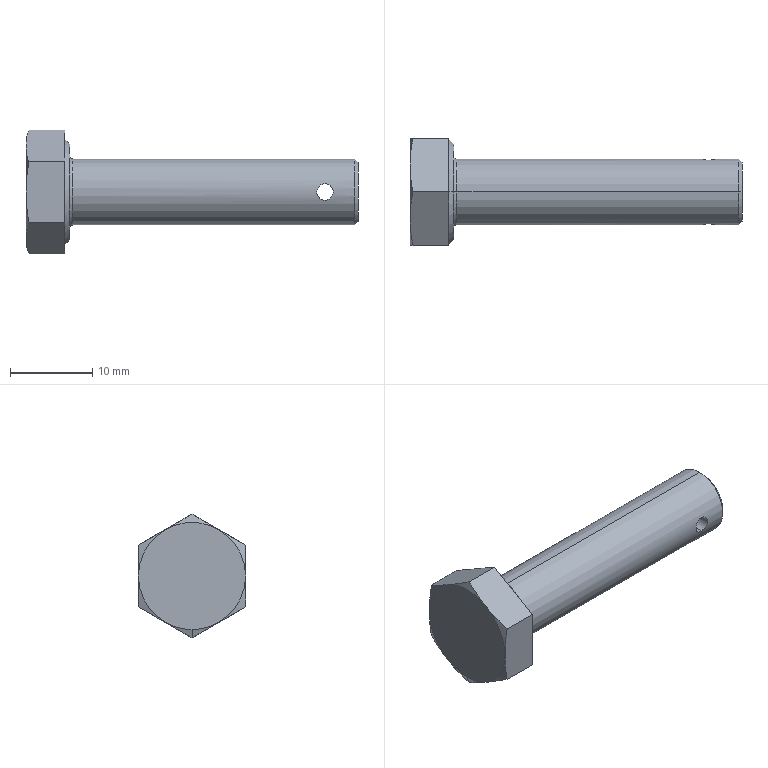Part | STEP file | hex bolts split pin hole-fine pitch-ab gb_PreviewCfg | 1 solid | 27 faces | box 40.3 x 13 x 15.011 mm | volume 2490 mm3 | cone 11 | plane 10 | cylinder 4 | torus 2 | commonest cylinder face diameters 2 x2 8 x2
STEP:
#1=CARTESIAN_POINT('',(5.7,0.,4.));
#2=VERTEX_POINT('',#1);
#3=CARTESIAN_POINT('',(5.7,0.,-4.));
#4=VERTEX_POINT('',#3);
#5=CARTESIAN_POINT('',(5.7,0.,0.));
#6=DIRECTION('',(1.,0.,0.));
#7=DIRECTION('',(0.,0.,-1.));
#8=AXIS2_PLACEMENT_3D('',#5,#6,#7);
#9=CIRCLE('',#8,4.);
#10=EDGE_CURVE('',#2,#4,#9,.T.);
#11=ORIENTED_EDGE('',*,*,#10,.F.);
#12=CARTESIAN_POINT('',(5.3,0.,4.4));
#13=VERTEX_POINT('',#12);
#14=CARTESIAN_POINT('',(5.7,0.,4.4));
#15=DIRECTION('',(0.,1.,0.));
#16=DIRECTION('',(0.,0.,1.));
#17=AXIS2_PLACEMENT_3D('',#14,#15,#16);
#18=CIRCLE('',#17,0.4);
#19=EDGE_CURVE('',#2,#13,#18,.T.);
#20=ORIENTED_EDGE('',*,*,#19,.T.);
#21=CARTESIAN_POINT('',(5.3,0.,-4.4));
#22=VERTEX_POINT('',#21);
#23=CARTESIAN_POINT('',(5.3,0.,0.));
#24=DIRECTION('',(-1.,0.,0.));
#25=DIRECTION('',(0.,0.,-1.));
#26=AXIS2_PLACEMENT_3D('',#23,#24,#25);
#27=CIRCLE('',#26,4.4);
#28=EDGE_CURVE('',#22,#13,#27,.T.);
#29=ORIENTED_EDGE('',*,*,#28,.F.);
#30=CARTESIAN_POINT('',(5.7,0.,-4.4));
#31=DIRECTION('',(0.,-1.,0.));
#32=DIRECTION('',(0.,0.,-1.));
#33=AXIS2_PLACEMENT_3D('',#30,#31,#32);
#34=CIRCLE('',#33,0.4);
#35=EDGE_CURVE('',#4,#22,#34,.T.);
#36=ORIENTED_EDGE('',*,*,#35,.F.);
#37=EDGE_LOOP('',(#11,#20,#29,#36));
#38=FACE_OUTER_BOUND('',#37,.T.);
#39=CARTESIAN_POINT('',(5.7,0.,0.));
#40=DIRECTION('',(1.,0.,0.));
#41=DIRECTION('',(0.,0.,-1.));
#42=AXIS2_PLACEMENT_3D('',#39,#40,#41);
#43=TOROIDAL_SURFACE('',#42,4.4,0.4);
#44=ADVANCED_FACE('',(#38),#43,.F.);
#45=CARTESIAN_POINT('',(36.3,-3.873,-1.));
#46=VERTEX_POINT('',#45);
#47=CARTESIAN_POINT('',(36.3,-3.873,1.));
#48=VERTEX_POINT('',#47);
#49=CARTESIAN_POINT('',(36.3,-3.873,-1.));
#50=CARTESIAN_POINT('',(36.169,-3.873,-1.));
#51=CARTESIAN_POINT('',(36.037,-3.88,-0.9736));
#52=CARTESIAN_POINT('',(35.796,-3.904,-0.8737));
#53=CARTESIAN_POINT('',(35.685,-3.92,-0.7996));
#54=CARTESIAN_POINT('',(35.501,-3.954,-0.6153));
#55=CARTESIAN_POINT('',(35.427,-3.97,-0.5057));
#56=CARTESIAN_POINT('',(35.326,-3.993,-0.2624));
#57=CARTESIAN_POINT('',(35.3,-4.,-0.1322));
#58=CARTESIAN_POINT('',(35.3,-4.,0.1316));
#59=CARTESIAN_POINT('',(35.326,-3.993,0.2627));
#60=CARTESIAN_POINT('',(35.426,-3.97,0.5039));
#61=CARTESIAN_POINT('',(35.501,-3.954,0.615));
#62=CARTESIAN_POINT('',(35.684,-3.921,0.7986));
#63=CARTESIAN_POINT('',(35.795,-3.904,0.873));
#64=CARTESIAN_POINT('',(36.036,-3.88,0.9733));
#65=CARTESIAN_POINT('',(36.167,-3.873,1.));
#66=CARTESIAN_POINT('',(36.3,-3.873,1.));
#67=B_SPLINE_CURVE_WITH_KNOTS('',3,(#49,#50,#51,#52,#53,#54,#55,#56,#57,#58,#59,#60,#61,#62,#63,#64,#65,#66),.UNSPECIFIED.,.F.,.F.,(4,2,2,2,2,2,2,2,4),(0.003139,0.003531,0.003923,0.004316,0.004708,0.0051,0.005492,0.005885,0.006277),.UNSPECIFIED.);
#68=EDGE_CURVE('',#46,#48,#67,.T.);
#69=ORIENTED_EDGE('',*,*,#68,.F.);
#70=CARTESIAN_POINT('',(36.3,3.873,-1.));
#71=VERTEX_POINT('',#70);
#72=CARTESIAN_POINT('',(36.3,-6.5,-1.));
#73=DIRECTION('',(0.,1.,0.));
#74=VECTOR('',#73,1000.);
#75=LINE('',#72,#74);
#76=EDGE_CURVE('',#46,#71,#75,.T.);
#77=ORIENTED_EDGE('',*,*,#76,.T.);
#78=CARTESIAN_POINT('',(36.3,3.873,1.));
#79=VERTEX_POINT('',#78);
#80=CARTESIAN_POINT('',(36.3,3.873,1.));
#81=CARTESIAN_POINT('',(36.167,3.873,1.));
#82=CARTESIAN_POINT('',(36.037,3.88,0.9737));
#83=CARTESIAN_POINT('',(35.795,3.904,0.8731));
#84=CARTESIAN_POINT('',(35.685,3.921,0.7988));
#85=CARTESIAN_POINT('',(35.501,3.954,0.6151));
#86=CARTESIAN_POINT('',(35.426,3.97,0.5039));
#87=CARTESIAN_POINT('',(35.327,3.993,0.2634));
#88=CARTESIAN_POINT('',(35.3,4.,0.1315));
#89=CARTESIAN_POINT('',(35.3,4.,-0.1306));
#90=CARTESIAN_POINT('',(35.326,3.993,-0.2619));
#91=CARTESIAN_POINT('',(35.427,3.97,-0.5048));
#92=CARTESIAN_POINT('',(35.5,3.954,-0.6147));
#93=CARTESIAN_POINT('',(35.686,3.92,-0.7999));
#94=CARTESIAN_POINT('',(35.796,3.904,-0.8735));
#95=CARTESIAN_POINT('',(36.037,3.88,-0.9737));
#96=CARTESIAN_POINT('',(36.169,3.873,-1.));
#97=CARTESIAN_POINT('',(36.3,3.873,-1.));
#98=B_SPLINE_CURVE_WITH_KNOTS('',3,(#80,#81,#82,#83,#84,#85,#86,#87,#88,#89,#90,#91,#92,#93,#94,#95,#96,#97),.UNSPECIFIED.,.F.,.F.,(4,2,2,2,2,2,2,2,4),(0.,0.0003924,0.0007847,0.001177,0.001569,0.001962,0.002354,0.002747,0.003139),.UNSPECIFIED.);
#99=EDGE_CURVE('',#79,#71,#98,.T.);
#100=ORIENTED_EDGE('',*,*,#99,.F.);
#101=CARTESIAN_POINT('',(36.3,-6.5,1.));
#102=DIRECTION('',(0.,1.,0.));
#103=VECTOR('',#102,1000.);
#104=LINE('',#101,#103);
#105=EDGE_CURVE('',#48,#79,#104,.T.);
#106=ORIENTED_EDGE('',*,*,#105,.F.);
#107=EDGE_LOOP('',(#69,#77,#100,#106));
#108=FACE_OUTER_BOUND('',#107,.T.);
#109=CARTESIAN_POINT('',(36.3,-6.5,0.));
#110=DIRECTION('',(0.,1.,0.));
#111=DIRECTION('',(0.,0.,1.));
#112=AXIS2_PLACEMENT_3D('',#109,#110,#111);
#113=CYLINDRICAL_SURFACE('',#112,1.);
#114=ADVANCED_FACE('',(#108),#113,.F.);
#115=CARTESIAN_POINT('',(40.3,0.,-3.6));
#116=VERTEX_POINT('',#115);
#117=CARTESIAN_POINT('',(40.3,0.,3.6));
#118=VERTEX_POINT('',#117);
#119=CARTESIAN_POINT('',(40.3,0.,0.));
#120=DIRECTION('',(1.,0.,0.));
#121=DIRECTION('',(0.,0.,-1.));
#122=AXIS2_PLACEMENT_3D('',#119,#120,#121);
#123=CIRCLE('',#122,3.6);
#124=EDGE_CURVE('',#116,#118,#123,.T.);
#125=ORIENTED_EDGE('',*,*,#124,.F.);
#126=CARTESIAN_POINT('',(39.9,0.,-4.));
#127=VERTEX_POINT('',#126);
#128=CARTESIAN_POINT('',(40.3,0.,-3.6));
#129=DIRECTION('',(-0.7071,0.,-0.7071));
#130=VECTOR('',#129,1000.);
#131=LINE('',#128,#130);
#132=EDGE_CURVE('',#116,#127,#131,.T.);
#133=ORIENTED_EDGE('',*,*,#132,.T.);
#134=CARTESIAN_POINT('',(39.9,0.,4.));
#135=VERTEX_POINT('',#134);
#136=CARTESIAN_POINT('',(39.9,0.,0.));
#137=DIRECTION('',(-1.,0.,0.));
#138=DIRECTION('',(0.,0.,-1.));
#139=AXIS2_PLACEMENT_3D('',#136,#137,#138);
#140=CIRCLE('',#139,4.);
#141=EDGE_CURVE('',#135,#127,#140,.T.);
#142=ORIENTED_EDGE('',*,*,#141,.F.);
#143=CARTESIAN_POINT('',(40.3,0.,3.6));
#144=DIRECTION('',(-0.7071,0.,0.7071));
#145=VECTOR('',#144,1000.);
#146=LINE('',#143,#145);
#147=EDGE_CURVE('',#118,#135,#146,.T.);
#148=ORIENTED_EDGE('',*,*,#147,.F.);
#149=EDGE_LOOP('',(#125,#133,#142,#148));
#150=FACE_OUTER_BOUND('',#149,.T.);
#151=CARTESIAN_POINT('',(40.3,0.,0.));
#152=DIRECTION('',(-1.,0.,0.));
#153=DIRECTION('',(0.,0.,1.));
#154=AXIS2_PLACEMENT_3D('',#151,#152,#153);
#155=CONICAL_SURFACE('',#154,3.6,0.7854);
#156=ADVANCED_FACE('',(#150),#155,.T.);
#157=ORIENTED_EDGE('',*,*,#99,.T.);
#158=CARTESIAN_POINT('',(36.3,3.873,-1.));
#159=CARTESIAN_POINT('',(36.431,3.873,-1.));
#160=CARTESIAN_POINT('',(36.563,3.88,-0.9736));
#161=CARTESIAN_POINT('',(36.804,3.904,-0.8737));
#162=CARTESIAN_POINT('',(36.915,3.92,-0.7996));
#163=CARTESIAN_POINT('',(37.099,3.954,-0.6153));
#164=CARTESIAN_POINT('',(37.173,3.97,-0.5057));
#165=CARTESIAN_POINT('',(37.274,3.993,-0.2624));
#166=CARTESIAN_POINT('',(37.3,4.,-0.1322));
#167=CARTESIAN_POINT('',(37.3,4.,0.1316));
#168=CARTESIAN_POINT('',(37.274,3.993,0.2627));
#169=CARTESIAN_POINT('',(37.174,3.97,0.5039));
#170=CARTESIAN_POINT('',(37.099,3.954,0.615));
#171=CARTESIAN_POINT('',(36.916,3.921,0.7986));
#172=CARTESIAN_POINT('',(36.805,3.904,0.873));
#173=CARTESIAN_POINT('',(36.564,3.88,0.9733));
#174=CARTESIAN_POINT('',(36.433,3.873,1.));
#175=CARTESIAN_POINT('',(36.3,3.873,1.));
#176=B_SPLINE_CURVE_WITH_KNOTS('',3,(#158,#159,#160,#161,#162,#163,#164,#165,#166,#167,#168,#169,#170,#171,#172,#173,#174,#175),.UNSPECIFIED.,.F.,.F.,(4,2,2,2,2,2,2,2,4),(0.003139,0.003531,0.003923,0.004316,0.004708,0.0051,0.005492,0.005885,0.006277),.UNSPECIFIED.);
#177=EDGE_CURVE('',#71,#79,#176,.T.);
#178=ORIENTED_EDGE('',*,*,#177,.T.);
#179=EDGE_LOOP('',(#157,#178));
#180=FACE_BOUND('',#179,.T.);
#181=ORIENTED_EDGE('',*,*,#141,.T.);
#182=CARTESIAN_POINT('',(40.3,0.,-4.));
#183=DIRECTION('',(-1.,0.,0.));
#184=VECTOR('',#183,1000.);
#185=LINE('',#182,#184);
#186=EDGE_CURVE('',#127,#4,#185,.T.);
#187=ORIENTED_EDGE('',*,*,#186,.T.);
#188=CARTESIAN_POINT('',(5.7,0.,0.));
#189=DIRECTION('',(1.,0.,0.));
#190=DIRECTION('',(0.,0.,-1.));
#191=AXIS2_PLACEMENT_3D('',#188,#189,#190);
#192=CIRCLE('',#191,4.);
#193=EDGE_CURVE('',#4,#2,#192,.T.);
#194=ORIENTED_EDGE('',*,*,#193,.T.);
#195=CARTESIAN_POINT('',(40.3,0.,4.));
#196=DIRECTION('',(-1.,0.,0.));
#197=VECTOR('',#196,1000.);
#198=LINE('',#195,#197);
#199=EDGE_CURVE('',#135,#2,#198,.T.);
#200=ORIENTED_EDGE('',*,*,#199,.F.);
#201=EDGE_LOOP('',(#181,#187,#194,#200));
#202=FACE_OUTER_BOUND('',#201,.T.);
#203=CARTESIAN_POINT('',(40.3,0.,0.));
#204=DIRECTION('',(-1.,0.,0.));
#205=DIRECTION('',(0.,0.,1.));
#206=AXIS2_PLACEMENT_3D('',#203,#204,#205);
#207=CYLINDRICAL_SURFACE('',#206,4.);
#208=ADVANCED_FACE('',(#180,#202),#207,.T.);
#209=CARTESIAN_POINT('',(0.,-3.25,-5.629));
#210=VERTEX_POINT('',#209);
#211=CARTESIAN_POINT('',(0.,0.,-6.5));
#212=VERTEX_POINT('',#211);
#213=CARTESIAN_POINT('',(0.,0.,0.));
#214=DIRECTION('',(1.,0.,0.));
#215=DIRECTION('',(0.,0.,-1.));
#216=AXIS2_PLACEMENT_3D('',#213,#214,#215);
#217=CIRCLE('',#216,6.5);
#218=EDGE_CURVE('',#210,#212,#217,.T.);
#219=ORIENTED_EDGE('',*,*,#218,.T.);
#220=CARTESIAN_POINT('',(0.366,0.,-7.506));
#221=VERTEX_POINT('',#220);
#222=CARTESIAN_POINT('',(0.,0.,-6.5));
#223=DIRECTION('',(0.342,0.,-0.9397));
#224=VECTOR('',#223,1000.);
#225=LINE('',#222,#224);
#226=EDGE_CURVE('',#212,#221,#225,.T.);
#227=ORIENTED_EDGE('',*,*,#226,.T.);
#228=CARTESIAN_POINT('',(0.366,0.,-7.506));
#229=CARTESIAN_POINT('',(0.2522,-0.5417,-7.193));
#230=CARTESIAN_POINT('',(0.1597,-1.083,-6.88));
#231=CARTESIAN_POINT('',(0.03346,-2.167,-6.255));
#232=CARTESIAN_POINT('',(0.,-2.708,-5.942));
#233=CARTESIAN_POINT('',(0.,-3.25,-5.629));
#234=B_SPLINE_CURVE_WITH_KNOTS('',3,(#228,#229,#230,#231,#232,#233),.UNSPECIFIED.,.F.,.F.,(4,2,4),(0.000000231,0.001877,0.003753),.UNSPECIFIED.);
#235=EDGE_CURVE('',#221,#210,#234,.T.);
#236=ORIENTED_EDGE('',*,*,#235,.T.);
#237=EDGE_LOOP('',(#219,#227,#236));
#238=FACE_OUTER_BOUND('',#237,.T.);
#239=CARTESIAN_POINT('',(0.,0.,0.));
#240=DIRECTION('',(1.,0.,0.));
#241=DIRECTION('',(0.,0.,-1.));
#242=AXIS2_PLACEMENT_3D('',#239,#240,#241);
#243=CONICAL_SURFACE('',#242,6.5,1.222);
#244=ADVANCED_FACE('',(#238),#243,.T.);
#245=CARTESIAN_POINT('',(5.3,0.,5.815));
#246=VERTEX_POINT('',#245);
#247=CARTESIAN_POINT('',(5.3,0.,-5.815));
#248=VERTEX_POINT('',#247);
#249=CARTESIAN_POINT('',(5.3,0.,0.));
#250=DIRECTION('',(-1.,0.,0.));
#251=DIRECTION('',(0.,0.,1.));
#252=AXIS2_PLACEMENT_3D('',#249,#250,#251);
#253=CIRCLE('',#252,5.815);
#254=EDGE_CURVE('',#246,#248,#253,.T.);
#255=ORIENTED_EDGE('',*,*,#254,.T.);
#256=CARTESIAN_POINT('',(4.7,0.,-6.415));
#257=VERTEX_POINT('',#256);
#258=CARTESIAN_POINT('',(4.7,0.,-6.415));
#259=DIRECTION('',(-0.7071,0.,-0.7071));
#260=VECTOR('',#259,1000.);
#261=LINE('',#258,#260);
#262=EDGE_CURVE('',#248,#257,#261,.T.);
#263=ORIENTED_EDGE('',*,*,#262,.T.);
#264=CARTESIAN_POINT('',(4.7,0.,6.415));
#265=VERTEX_POINT('',#264);
#266=CARTESIAN_POINT('',(4.7,0.,0.));
#267=DIRECTION('',(-1.,0.,0.));
#268=DIRECTION('',(0.,0.,1.));
#269=AXIS2_PLACEMENT_3D('',#266,#267,#268);
#270=CIRCLE('',#269,6.415);
#271=EDGE_CURVE('',#265,#257,#270,.T.);
#272=ORIENTED_EDGE('',*,*,#271,.F.);
#273=CARTESIAN_POINT('',(4.7,0.,6.415));
#274=DIRECTION('',(-0.7071,0.,0.7071));
#275=VECTOR('',#274,1000.);
#276=LINE('',#273,#275);
#277=EDGE_CURVE('',#246,#265,#276,.T.);
#278=ORIENTED_EDGE('',*,*,#277,.F.);
#279=EDGE_LOOP('',(#255,#263,#272,#278));
#280=FACE_OUTER_BOUND('',#279,.T.);
#281=CARTESIAN_POINT('',(4.7,0.,0.));
#282=DIRECTION('',(-1.,0.,0.));
#283=DIRECTION('',(0.,0.,1.));
#284=AXIS2_PLACEMENT_3D('',#281,#282,#283);
#285=CONICAL_SURFACE('',#284,6.415,0.7854);
#286=ADVANCED_FACE('',(#280),#285,.T.);
#287=ORIENTED_EDGE('',*,*,#28,.T.);
#288=CARTESIAN_POINT('',(5.3,0.,0.));
#289=DIRECTION('',(-1.,0.,0.));
#290=DIRECTION('',(0.,0.,-1.));
#291=AXIS2_PLACEMENT_3D('',#288,#289,#290);
#292=CIRCLE('',#291,4.4);
#293=EDGE_CURVE('',#13,#22,#292,.T.);
#294=ORIENTED_EDGE('',*,*,#293,.T.);
#295=EDGE_LOOP('',(#287,#294));
#296=FACE_BOUND('',#295,.T.);
#297=ORIENTED_EDGE('',*,*,#254,.F.);
#298=CARTESIAN_POINT('',(5.3,0.,0.));
#299=DIRECTION('',(-1.,0.,0.));
#300=DIRECTION('',(0.,0.,1.));
#301=AXIS2_PLACEMENT_3D('',#298,#299,#300);
#302=CIRCLE('',#301,5.815);
#303=EDGE_CURVE('',#248,#246,#302,.T.);
#304=ORIENTED_EDGE('',*,*,#303,.F.);
#305=EDGE_LOOP('',(#297,#304));
#306=FACE_OUTER_BOUND('',#305,.T.);
#307=CARTESIAN_POINT('',(5.3,0.,-7.506));
#308=DIRECTION('',(1.,0.,0.));
#309=DIRECTION('',(0.,0.,-1.));
#310=AXIS2_PLACEMENT_3D('',#307,#308,#309);
#311=PLANE('',#310);
#312=ADVANCED_FACE('',(#296,#306),#311,.T.);
#313=ORIENTED_EDGE('',*,*,#235,.F.);
#314=CARTESIAN_POINT('',(4.7,0.,-7.506));
#315=VERTEX_POINT('',#314);
#316=CARTESIAN_POINT('',(5.3,0.,-7.506));
#317=DIRECTION('',(-1.,0.,0.));
#318=VECTOR('',#317,1000.);
#319=LINE('',#316,#318);
#320=EDGE_CURVE('',#315,#221,#319,.T.);
#321=ORIENTED_EDGE('',*,*,#320,.F.);
#322=CARTESIAN_POINT('',(4.7,-6.5,-3.753));
#323=VERTEX_POINT('',#322);
#324=CARTESIAN_POINT('',(4.7,-6.5,-3.753));
#325=DIRECTION('',(0.,0.866,-0.5));
#326=VECTOR('',#325,1000.);
#327=LINE('',#324,#326);
#328=EDGE_CURVE('',#323,#315,#327,.T.);
#329=ORIENTED_EDGE('',*,*,#328,.F.);
#330=CARTESIAN_POINT('',(0.366,-6.5,-3.753));
#331=VERTEX_POINT('',#330);
#332=CARTESIAN_POINT('',(5.3,-6.5,-3.753));
#333=DIRECTION('',(-1.,0.,0.));
#334=VECTOR('',#333,1000.);
#335=LINE('',#332,#334);
#336=EDGE_CURVE('',#323,#331,#335,.T.);
#337=ORIENTED_EDGE('',*,*,#336,.T.);
#338=CARTESIAN_POINT('',(0.,-3.25,-5.629));
#339=CARTESIAN_POINT('',(0.,-3.792,-5.316));
#340=CARTESIAN_POINT('',(0.03346,-4.333,-5.004));
#341=CARTESIAN_POINT('',(0.1597,-5.417,-4.378));
#342=CARTESIAN_POINT('',(0.2522,-5.958,-4.066));
#343=CARTESIAN_POINT('',(0.366,-6.5,-3.753));
#344=B_SPLINE_CURVE_WITH_KNOTS('',3,(#338,#339,#340,#341,#342,#343),.UNSPECIFIED.,.F.,.F.,(4,2,4),(0.003753,0.005629,0.007506),.UNSPECIFIED.);
#345=EDGE_CURVE('',#210,#331,#344,.T.);
#346=ORIENTED_EDGE('',*,*,#345,.F.);
#347=EDGE_LOOP('',(#313,#321,#329,#337,#346));
#348=FACE_OUTER_BOUND('',#347,.T.);
#349=CARTESIAN_POINT('',(5.3,-6.5,-3.753));
#350=DIRECTION('',(0.,0.5,0.866));
#351=DIRECTION('',(0.,-0.866,0.5));
#352=AXIS2_PLACEMENT_3D('',#349,#350,#351);
#353=PLANE('',#352);
#354=ADVANCED_FACE('',(#348),#353,.F.);
#355=CARTESIAN_POINT('',(0.366,6.5,-3.753));
#356=VERTEX_POINT('',#355);
#357=CARTESIAN_POINT('',(0.,3.25,-5.629));
#358=VERTEX_POINT('',#357);
#359=CARTESIAN_POINT('',(0.366,6.5,-3.753));
#360=CARTESIAN_POINT('',(0.2522,5.958,-4.066));
#361=CARTESIAN_POINT('',(0.1597,5.417,-4.378));
#362=CARTESIAN_POINT('',(0.03346,4.333,-5.004));
#363=CARTESIAN_POINT('',(0.,3.792,-5.316));
#364=CARTESIAN_POINT('',(0.,3.25,-5.629));
#365=B_SPLINE_CURVE_WITH_KNOTS('',3,(#359,#360,#361,#362,#363,#364),.UNSPECIFIED.,.F.,.F.,(4,2,4),(0.000000231,0.001877,0.003753),.UNSPECIFIED.);
#366=EDGE_CURVE('',#356,#358,#365,.T.);
#367=ORIENTED_EDGE('',*,*,#366,.F.);
#368=CARTESIAN_POINT('',(4.7,6.5,-3.753));
#369=VERTEX_POINT('',#368);
#370=CARTESIAN_POINT('',(5.3,6.5,-3.753));
#371=DIRECTION('',(-1.,0.,0.));
#372=VECTOR('',#371,1000.);
#373=LINE('',#370,#372);
#374=EDGE_CURVE('',#369,#356,#373,.T.);
#375=ORIENTED_EDGE('',*,*,#374,.F.);
#376=CARTESIAN_POINT('',(4.7,0.,-7.506));
#377=DIRECTION('',(0.,0.866,0.5));
#378=VECTOR('',#377,1000.);
#379=LINE('',#376,#378);
#380=EDGE_CURVE('',#315,#369,#379,.T.);
#381=ORIENTED_EDGE('',*,*,#380,.F.);
#382=ORIENTED_EDGE('',*,*,#320,.T.);
#383=CARTESIAN_POINT('',(0.,3.25,-5.629));
#384=CARTESIAN_POINT('',(0.,2.708,-5.942));
#385=CARTESIAN_POINT('',(0.03346,2.167,-6.255));
#386=CARTESIAN_POINT('',(0.1597,1.083,-6.88));
#387=CARTESIAN_POINT('',(0.2522,0.5417,-7.193));
#388=CARTESIAN_POINT('',(0.366,0.,-7.506));
#389=B_SPLINE_CURVE_WITH_KNOTS('',3,(#383,#384,#385,#386,#387,#388),.UNSPECIFIED.,.F.,.F.,(4,2,4),(0.003753,0.005629,0.007506),.UNSPECIFIED.);
#390=EDGE_CURVE('',#358,#221,#389,.T.);
#391=ORIENTED_EDGE('',*,*,#390,.F.);
#392=EDGE_LOOP('',(#367,#375,#381,#382,#391));
#393=FACE_OUTER_BOUND('',#392,.T.);
#394=CARTESIAN_POINT('',(5.3,0.,-7.506));
#395=DIRECTION('',(0.,-0.5,0.866));
#396=DIRECTION('',(0.,-0.866,-0.5));
#397=AXIS2_PLACEMENT_3D('',#394,#395,#396);
#398=PLANE('',#397);
#399=ADVANCED_FACE('',(#393),#398,.F.);
#400=CARTESIAN_POINT('',(0.366,6.5,3.753));
#401=VERTEX_POINT('',#400);
#402=CARTESIAN_POINT('',(0.,6.5,0.));
#403=VERTEX_POINT('',#402);
#404=CARTESIAN_POINT('',(0.366,6.5,3.753));
#405=CARTESIAN_POINT('',(0.2525,6.5,3.129));
#406=CARTESIAN_POINT('',(0.16,6.5,2.504));
#407=CARTESIAN_POINT('',(0.0336,6.5,1.253));
#408=CARTESIAN_POINT('',(0.,6.5,0.6268));
#409=CARTESIAN_POINT('',(0.,6.5,0.));
#410=B_SPLINE_CURVE_WITH_KNOTS('',3,(#404,#405,#406,#407,#408,#409),.UNSPECIFIED.,.F.,.F.,(4,2,4),(0.01353,0.01542,0.01732),.UNSPECIFIED.);
#411=EDGE_CURVE('',#401,#403,#410,.T.);
#412=ORIENTED_EDGE('',*,*,#411,.F.);
#413=CARTESIAN_POINT('',(4.7,6.5,3.753));
#414=VERTEX_POINT('',#413);
#415=CARTESIAN_POINT('',(5.3,6.5,3.753));
#416=DIRECTION('',(-1.,0.,0.));
#417=VECTOR('',#416,1000.);
#418=LINE('',#415,#417);
#419=EDGE_CURVE('',#414,#401,#418,.T.);
#420=ORIENTED_EDGE('',*,*,#419,.F.);
#421=CARTESIAN_POINT('',(4.7,6.5,-3.753));
#422=DIRECTION('',(0.,0.,1.));
#423=VECTOR('',#422,1000.);
#424=LINE('',#421,#423);
#425=EDGE_CURVE('',#369,#414,#424,.T.);
#426=ORIENTED_EDGE('',*,*,#425,.F.);
#427=ORIENTED_EDGE('',*,*,#374,.T.);
#428=CARTESIAN_POINT('',(0.,6.5,0.));
#429=CARTESIAN_POINT('',(0.,6.5,-0.625));
#430=CARTESIAN_POINT('',(0.03342,6.5,-1.251));
#431=CARTESIAN_POINT('',(0.1599,6.5,-2.503));
#432=CARTESIAN_POINT('',(0.2529,6.5,-3.131));
#433=CARTESIAN_POINT('',(0.366,6.5,-3.753));
#434=B_SPLINE_CURVE_WITH_KNOTS('',3,(#428,#429,#430,#431,#432,#433),.UNSPECIFIED.,.F.,.F.,(4,2,4),(0.01732,0.0192,0.02109),.UNSPECIFIED.);
#435=EDGE_CURVE('',#403,#356,#434,.T.);
#436=ORIENTED_EDGE('',*,*,#435,.F.);
#437=EDGE_LOOP('',(#412,#420,#426,#427,#436));
#438=FACE_OUTER_BOUND('',#437,.T.);
#439=CARTESIAN_POINT('',(5.3,6.5,-3.753));
#440=DIRECTION('',(0.,-1.,0.));
#441=DIRECTION('',(0.,0.,-1.));
#442=AXIS2_PLACEMENT_3D('',#439,#440,#441);
#443=PLANE('',#442);
#444=ADVANCED_FACE('',(#438),#443,.F.);
#445=CARTESIAN_POINT('',(0.366,0.,7.506));
#446=VERTEX_POINT('',#445);
#447=CARTESIAN_POINT('',(0.,3.25,5.629));
#448=VERTEX_POINT('',#447);
#449=CARTESIAN_POINT('',(0.366,0.,7.506));
#450=CARTESIAN_POINT('',(0.2522,0.5417,7.193));
#451=CARTESIAN_POINT('',(0.1597,1.083,6.88));
#452=CARTESIAN_POINT('',(0.03346,2.167,6.255));
#453=CARTESIAN_POINT('',(0.,2.708,5.942));
#454=CARTESIAN_POINT('',(0.,3.25,5.629));
#455=B_SPLINE_CURVE_WITH_KNOTS('',3,(#449,#450,#451,#452,#453,#454),.UNSPECIFIED.,.F.,.F.,(4,2,4),(0.000000231,0.001877,0.003753),.UNSPECIFIED.);
#456=EDGE_CURVE('',#446,#448,#455,.T.);
#457=ORIENTED_EDGE('',*,*,#456,.F.);
#458=CARTESIAN_POINT('',(4.7,0.,7.506));
#459=VERTEX_POINT('',#458);
#460=CARTESIAN_POINT('',(5.3,0.,7.506));
#461=DIRECTION('',(-1.,0.,0.));
#462=VECTOR('',#461,1000.);
#463=LINE('',#460,#462);
#464=EDGE_CURVE('',#459,#446,#463,.T.);
#465=ORIENTED_EDGE('',*,*,#464,.F.);
#466=CARTESIAN_POINT('',(4.7,6.5,3.753));
#467=DIRECTION('',(0.,-0.866,0.5));
#468=VECTOR('',#467,1000.);
#469=LINE('',#466,#468);
#470=EDGE_CURVE('',#414,#459,#469,.T.);
#471=ORIENTED_EDGE('',*,*,#470,.F.);
#472=ORIENTED_EDGE('',*,*,#419,.T.);
#473=CARTESIAN_POINT('',(0.,3.25,5.629));
#474=CARTESIAN_POINT('',(0.,3.792,5.316));
#475=CARTESIAN_POINT('',(0.03346,4.333,5.004));
#476=CARTESIAN_POINT('',(0.1597,5.417,4.378));
#477=CARTESIAN_POINT('',(0.2522,5.958,4.066));
#478=CARTESIAN_POINT('',(0.366,6.5,3.753));
#479=B_SPLINE_CURVE_WITH_KNOTS('',3,(#473,#474,#475,#476,#477,#478),.UNSPECIFIED.,.F.,.F.,(4,2,4),(0.003753,0.005629,0.007506),.UNSPECIFIED.);
#480=EDGE_CURVE('',#448,#401,#479,.T.);
#481=ORIENTED_EDGE('',*,*,#480,.F.);
#482=EDGE_LOOP('',(#457,#465,#471,#472,#481));
#483=FACE_OUTER_BOUND('',#482,.T.);
#484=CARTESIAN_POINT('',(5.3,6.5,3.753));
#485=DIRECTION('',(0.,-0.5,-0.866));
#486=DIRECTION('',(0.,0.866,-0.5));
#487=AXIS2_PLACEMENT_3D('',#484,#485,#486);
#488=PLANE('',#487);
#489=ADVANCED_FACE('',(#483),#488,.F.);
#490=CARTESIAN_POINT('',(0.366,-6.5,3.753));
#491=VERTEX_POINT('',#490);
#492=CARTESIAN_POINT('',(0.,-3.25,5.629));
#493=VERTEX_POINT('',#492);
#494=CARTESIAN_POINT('',(0.366,-6.5,3.753));
#495=CARTESIAN_POINT('',(0.2522,-5.958,4.066));
#496=CARTESIAN_POINT('',(0.1597,-5.417,4.378));
#497=CARTESIAN_POINT('',(0.03346,-4.333,5.004));
#498=CARTESIAN_POINT('',(0.,-3.792,5.316));
#499=CARTESIAN_POINT('',(0.,-3.25,5.629));
#500=B_SPLINE_CURVE_WITH_KNOTS('',3,(#494,#495,#496,#497,#498,#499),.UNSPECIFIED.,.F.,.F.,(4,2,4),(0.000000231,0.001877,0.003753),.UNSPECIFIED.);
#501=EDGE_CURVE('',#491,#493,#500,.T.);
#502=ORIENTED_EDGE('',*,*,#501,.F.);
#503=CARTESIAN_POINT('',(4.7,-6.5,3.753));
#504=VERTEX_POINT('',#503);
#505=CARTESIAN_POINT('',(5.3,-6.5,3.753));
#506=DIRECTION('',(-1.,0.,0.));
#507=VECTOR('',#506,1000.);
#508=LINE('',#505,#507);
#509=EDGE_CURVE('',#504,#491,#508,.T.);
#510=ORIENTED_EDGE('',*,*,#509,.F.);
#511=CARTESIAN_POINT('',(4.7,0.,7.506));
#512=DIRECTION('',(0.,-0.866,-0.5));
#513=VECTOR('',#512,1000.);
#514=LINE('',#511,#513);
#515=EDGE_CURVE('',#459,#504,#514,.T.);
#516=ORIENTED_EDGE('',*,*,#515,.F.);
#517=ORIENTED_EDGE('',*,*,#464,.T.);
#518=CARTESIAN_POINT('',(0.,-3.25,5.629));
#519=CARTESIAN_POINT('',(0.,-2.708,5.942));
#520=CARTESIAN_POINT('',(0.03346,-2.167,6.255));
#521=CARTESIAN_POINT('',(0.1597,-1.083,6.88));
#522=CARTESIAN_POINT('',(0.2522,-0.5417,7.193));
#523=CARTESIAN_POINT('',(0.366,0.,7.506));
#524=B_SPLINE_CURVE_WITH_KNOTS('',3,(#518,#519,#520,#521,#522,#523),.UNSPECIFIED.,.F.,.F.,(4,2,4),(0.003753,0.005629,0.007506),.UNSPECIFIED.);
#525=EDGE_CURVE('',#493,#446,#524,.T.);
#526=ORIENTED_EDGE('',*,*,#525,.F.);
#527=EDGE_LOOP('',(#502,#510,#516,#517,#526));
#528=FACE_OUTER_BOUND('',#527,.T.);
#529=CARTESIAN_POINT('',(5.3,0.,7.506));
#530=DIRECTION('',(0.,0.5,-0.866));
#531=DIRECTION('',(0.,0.866,0.5));
#532=AXIS2_PLACEMENT_3D('',#529,#530,#531);
#533=PLANE('',#532);
#534=ADVANCED_FACE('',(#528),#533,.F.);
#535=CARTESIAN_POINT('',(0.,-6.5,0.));
#536=VERTEX_POINT('',#535);
#537=CARTESIAN_POINT('',(0.366,-6.5,-3.753));
#538=CARTESIAN_POINT('',(0.2529,-6.5,-3.131));
#539=CARTESIAN_POINT('',(0.1599,-6.5,-2.503));
#540=CARTESIAN_POINT('',(0.03342,-6.5,-1.251));
#541=CARTESIAN_POINT('',(0.,-6.5,-0.625));
#542=CARTESIAN_POINT('',(0.,-6.5,0.));
#543=B_SPLINE_CURVE_WITH_KNOTS('',3,(#537,#538,#539,#540,#541,#542),.UNSPECIFIED.,.F.,.F.,(4,2,4),(0.006384,0.008275,0.01017),.UNSPECIFIED.);
#544=EDGE_CURVE('',#331,#536,#543,.T.);
#545=ORIENTED_EDGE('',*,*,#544,.F.);
#546=ORIENTED_EDGE('',*,*,#336,.F.);
#547=CARTESIAN_POINT('',(4.7,-6.5,3.753));
#548=DIRECTION('',(0.,0.,-1.));
#549=VECTOR('',#548,1000.);
#550=LINE('',#547,#549);
#551=EDGE_CURVE('',#504,#323,#550,.T.);
#552=ORIENTED_EDGE('',*,*,#551,.F.);
#553=ORIENTED_EDGE('',*,*,#509,.T.);
#554=CARTESIAN_POINT('',(0.,-6.5,0.));
#555=CARTESIAN_POINT('',(0.,-6.5,0.6268));
#556=CARTESIAN_POINT('',(0.0336,-6.5,1.253));
#557=CARTESIAN_POINT('',(0.16,-6.5,2.504));
#558=CARTESIAN_POINT('',(0.2525,-6.5,3.129));
#559=CARTESIAN_POINT('',(0.366,-6.5,3.753));
#560=B_SPLINE_CURVE_WITH_KNOTS('',3,(#554,#555,#556,#557,#558,#559),.UNSPECIFIED.,.F.,.F.,(4,2,4),(0.01017,0.01206,0.01396),.UNSPECIFIED.);
#561=EDGE_CURVE('',#536,#491,#560,.T.);
#562=ORIENTED_EDGE('',*,*,#561,.F.);
#563=EDGE_LOOP('',(#545,#546,#552,#553,#562));
#564=FACE_OUTER_BOUND('',#563,.T.);
#565=CARTESIAN_POINT('',(5.3,-6.5,3.753));
#566=DIRECTION('',(0.,1.,0.));
#567=DIRECTION('',(0.,0.,1.));
#568=AXIS2_PLACEMENT_3D('',#565,#566,#567);
#569=PLANE('',#568);
#570=ADVANCED_FACE('',(#564),#569,.F.);
#571=ORIENTED_EDGE('',*,*,#271,.T.);
#572=CARTESIAN_POINT('',(4.7,0.,0.));
#573=DIRECTION('',(-1.,0.,0.));
#574=DIRECTION('',(0.,0.,1.));
#575=AXIS2_PLACEMENT_3D('',#572,#573,#574);
#576=CIRCLE('',#575,6.415);
#577=EDGE_CURVE('',#257,#265,#576,.T.);
#578=ORIENTED_EDGE('',*,*,#577,.T.);
#579=EDGE_LOOP('',(#571,#578));
#580=FACE_BOUND('',#579,.T.);
#581=ORIENTED_EDGE('',*,*,#328,.T.);
#582=ORIENTED_EDGE('',*,*,#380,.T.);
#583=ORIENTED_EDGE('',*,*,#425,.T.);
#584=ORIENTED_EDGE('',*,*,#470,.T.);
#585=ORIENTED_EDGE('',*,*,#515,.T.);
#586=ORIENTED_EDGE('',*,*,#551,.T.);
#587=EDGE_LOOP('',(#581,#582,#583,#584,#585,#586));
#588=FACE_OUTER_BOUND('',#587,.T.);
#589=CARTESIAN_POINT('',(4.7,0.,-6.415));
#590=DIRECTION('',(1.,0.,0.));
#591=DIRECTION('',(0.,0.,-1.));
#592=AXIS2_PLACEMENT_3D('',#589,#590,#591);
#593=PLANE('',#592);
#594=ADVANCED_FACE('',(#580,#588),#593,.T.);
#595=ORIENTED_EDGE('',*,*,#262,.F.);
#596=ORIENTED_EDGE('',*,*,#303,.T.);
#597=ORIENTED_EDGE('',*,*,#277,.T.);
#598=ORIENTED_EDGE('',*,*,#577,.F.);
#599=EDGE_LOOP('',(#595,#596,#597,#598));
#600=FACE_OUTER_BOUND('',#599,.T.);
#601=CARTESIAN_POINT('',(4.7,0.,0.));
#602=DIRECTION('',(-1.,0.,0.));
#603=DIRECTION('',(0.,0.,1.));
#604=AXIS2_PLACEMENT_3D('',#601,#602,#603);
#605=CONICAL_SURFACE('',#604,6.415,0.7854);
#606=ADVANCED_FACE('',(#600),#605,.T.);
#607=ORIENTED_EDGE('',*,*,#226,.F.);
#608=CARTESIAN_POINT('',(0.,0.,0.));
#609=DIRECTION('',(1.,0.,0.));
#610=DIRECTION('',(0.,0.,-1.));
#611=AXIS2_PLACEMENT_3D('',#608,#609,#610);
#612=CIRCLE('',#611,6.5);
#613=EDGE_CURVE('',#212,#358,#612,.T.);
#614=ORIENTED_EDGE('',*,*,#613,.T.);
#615=ORIENTED_EDGE('',*,*,#390,.T.);
#616=EDGE_LOOP('',(#607,#614,#615));
#617=FACE_OUTER_BOUND('',#616,.T.);
#618=CARTESIAN_POINT('',(0.,0.,0.));
#619=DIRECTION('',(1.,0.,0.));
#620=DIRECTION('',(0.,0.,-1.));
#621=AXIS2_PLACEMENT_3D('',#618,#619,#620);
#622=CONICAL_SURFACE('',#621,6.5,1.222);
#623=ADVANCED_FACE('',(#617),#622,.T.);
#624=ORIENTED_EDGE('',*,*,#345,.T.);
#625=ORIENTED_EDGE('',*,*,#544,.T.);
#626=CARTESIAN_POINT('',(0.,0.,0.));
#627=DIRECTION('',(1.,0.,0.));
#628=DIRECTION('',(0.,0.,-1.));
#629=AXIS2_PLACEMENT_3D('',#626,#627,#628);
#630=CIRCLE('',#629,6.5);
#631=EDGE_CURVE('',#536,#210,#630,.T.);
#632=ORIENTED_EDGE('',*,*,#631,.T.);
#633=EDGE_LOOP('',(#624,#625,#632));
#634=FACE_OUTER_BOUND('',#633,.T.);
#635=CARTESIAN_POINT('',(0.,0.,0.));
#636=DIRECTION('',(1.,0.,0.));
#637=DIRECTION('',(0.,0.,-1.));
#638=AXIS2_PLACEMENT_3D('',#635,#636,#637);
#639=CONICAL_SURFACE('',#638,6.5,1.222);
#640=ADVANCED_FACE('',(#634),#639,.T.);
#641=ORIENTED_EDGE('',*,*,#501,.T.);
#642=CARTESIAN_POINT('',(0.,0.,0.));
#643=DIRECTION('',(1.,0.,0.));
#644=DIRECTION('',(0.,0.,-1.));
#645=AXIS2_PLACEMENT_3D('',#642,#643,#644);
#646=CIRCLE('',#645,6.5);
#647=EDGE_CURVE('',#493,#536,#646,.T.);
#648=ORIENTED_EDGE('',*,*,#647,.T.);
#649=ORIENTED_EDGE('',*,*,#561,.T.);
#650=EDGE_LOOP('',(#641,#648,#649));
#651=FACE_OUTER_BOUND('',#650,.T.);
#652=CARTESIAN_POINT('',(0.,0.,0.));
#653=DIRECTION('',(1.,0.,0.));
#654=DIRECTION('',(0.,0.,-1.));
#655=AXIS2_PLACEMENT_3D('',#652,#653,#654);
#656=CONICAL_SURFACE('',#655,6.5,1.222);
#657=ADVANCED_FACE('',(#651),#656,.T.);
#658=ORIENTED_EDGE('',*,*,#456,.T.);
#659=CARTESIAN_POINT('',(0.,0.,0.));
#660=DIRECTION('',(1.,0.,0.));
#661=DIRECTION('',(0.,0.,-1.));
#662=AXIS2_PLACEMENT_3D('',#659,#660,#661);
#663=CIRCLE('',#662,6.5);
#664=EDGE_CURVE('',#448,#493,#663,.T.);
#665=ORIENTED_EDGE('',*,*,#664,.T.);
#666=ORIENTED_EDGE('',*,*,#525,.T.);
#667=EDGE_LOOP('',(#658,#665,#666));
#668=FACE_OUTER_BOUND('',#667,.T.);
#669=CARTESIAN_POINT('',(0.,0.,0.));
#670=DIRECTION('',(1.,0.,0.));
#671=DIRECTION('',(0.,0.,-1.));
#672=AXIS2_PLACEMENT_3D('',#669,#670,#671);
#673=CONICAL_SURFACE('',#672,6.5,1.222);
#674=ADVANCED_FACE('',(#668),#673,.T.);
#675=ORIENTED_EDGE('',*,*,#411,.T.);
#676=CARTESIAN_POINT('',(0.,0.,0.));
#677=DIRECTION('',(-1.,0.,0.));
#678=DIRECTION('',(0.,0.,1.));
#679=AXIS2_PLACEMENT_3D('',#676,#677,#678);
#680=CIRCLE('',#679,6.5);
#681=EDGE_CURVE('',#448,#403,#680,.T.);
#682=ORIENTED_EDGE('',*,*,#681,.F.);
#683=ORIENTED_EDGE('',*,*,#480,.T.);
#684=EDGE_LOOP('',(#675,#682,#683));
#685=FACE_OUTER_BOUND('',#684,.T.);
#686=CARTESIAN_POINT('',(0.,0.,0.));
#687=DIRECTION('',(1.,0.,0.));
#688=DIRECTION('',(0.,0.,-1.));
#689=AXIS2_PLACEMENT_3D('',#686,#687,#688);
#690=CONICAL_SURFACE('',#689,6.5,1.222);
#691=ADVANCED_FACE('',(#685),#690,.T.);
#692=ORIENTED_EDGE('',*,*,#435,.T.);
#693=ORIENTED_EDGE('',*,*,#366,.T.);
#694=CARTESIAN_POINT('',(0.,0.,0.));
#695=DIRECTION('',(1.,0.,0.));
#696=DIRECTION('',(0.,0.,-1.));
#697=AXIS2_PLACEMENT_3D('',#694,#695,#696);
#698=CIRCLE('',#697,6.5);
#699=EDGE_CURVE('',#358,#403,#698,.T.);
#700=ORIENTED_EDGE('',*,*,#699,.T.);
#701=EDGE_LOOP('',(#692,#693,#700));
#702=FACE_OUTER_BOUND('',#701,.T.);
#703=CARTESIAN_POINT('',(0.,0.,0.));
#704=DIRECTION('',(1.,0.,0.));
#705=DIRECTION('',(0.,0.,-1.));
#706=AXIS2_PLACEMENT_3D('',#703,#704,#705);
#707=CONICAL_SURFACE('',#706,6.5,1.222);
#708=ADVANCED_FACE('',(#702),#707,.T.);
#709=ORIENTED_EDGE('',*,*,#699,.F.);
#710=ORIENTED_EDGE('',*,*,#613,.F.);
#711=ORIENTED_EDGE('',*,*,#218,.F.);
#712=ORIENTED_EDGE('',*,*,#631,.F.);
#713=ORIENTED_EDGE('',*,*,#647,.F.);
#714=ORIENTED_EDGE('',*,*,#664,.F.);
#715=ORIENTED_EDGE('',*,*,#681,.T.);
#716=EDGE_LOOP('',(#709,#710,#711,#712,#713,#714,#715));
#717=FACE_OUTER_BOUND('',#716,.T.);
#718=CARTESIAN_POINT('',(0.,0.,-7.506));
#719=DIRECTION('',(1.,0.,0.));
#720=DIRECTION('',(0.,0.,-1.));
#721=AXIS2_PLACEMENT_3D('',#718,#719,#720);
#722=PLANE('',#721);
#723=ADVANCED_FACE('',(#717),#722,.F.);
#724=ORIENTED_EDGE('',*,*,#186,.F.);
#725=CARTESIAN_POINT('',(39.9,0.,0.));
#726=DIRECTION('',(-1.,0.,0.));
#727=DIRECTION('',(0.,0.,-1.));
#728=AXIS2_PLACEMENT_3D('',#725,#726,#727);
#729=CIRCLE('',#728,4.);
#730=EDGE_CURVE('',#127,#135,#729,.T.);
#731=ORIENTED_EDGE('',*,*,#730,.T.);
#732=ORIENTED_EDGE('',*,*,#199,.T.);
#733=ORIENTED_EDGE('',*,*,#10,.T.);
#734=EDGE_LOOP('',(#724,#731,#732,#733));
#735=FACE_OUTER_BOUND('',#734,.T.);
#736=CARTESIAN_POINT('',(36.3,-3.873,1.));
#737=CARTESIAN_POINT('',(36.433,-3.873,1.));
#738=CARTESIAN_POINT('',(36.563,-3.88,0.9737));
#739=CARTESIAN_POINT('',(36.805,-3.904,0.8731));
#740=CARTESIAN_POINT('',(36.915,-3.921,0.7988));
#741=CARTESIAN_POINT('',(37.099,-3.954,0.6151));
#742=CARTESIAN_POINT('',(37.174,-3.97,0.5039));
#743=CARTESIAN_POINT('',(37.273,-3.993,0.2634));
#744=CARTESIAN_POINT('',(37.3,-4.,0.1315));
#745=CARTESIAN_POINT('',(37.3,-4.,-0.1306));
#746=CARTESIAN_POINT('',(37.274,-3.993,-0.2619));
#747=CARTESIAN_POINT('',(37.173,-3.97,-0.5048));
#748=CARTESIAN_POINT('',(37.1,-3.954,-0.6147));
#749=CARTESIAN_POINT('',(36.914,-3.92,-0.7999));
#750=CARTESIAN_POINT('',(36.804,-3.904,-0.8735));
#751=CARTESIAN_POINT('',(36.563,-3.88,-0.9737));
#752=CARTESIAN_POINT('',(36.431,-3.873,-1.));
#753=CARTESIAN_POINT('',(36.3,-3.873,-1.));
#754=B_SPLINE_CURVE_WITH_KNOTS('',3,(#736,#737,#738,#739,#740,#741,#742,#743,#744,#745,#746,#747,#748,#749,#750,#751,#752,#753),.UNSPECIFIED.,.F.,.F.,(4,2,2,2,2,2,2,2,4),(0.,0.0003924,0.0007847,0.001177,0.001569,0.001962,0.002354,0.002747,0.003139),.UNSPECIFIED.);
#755=EDGE_CURVE('',#48,#46,#754,.T.);
#756=ORIENTED_EDGE('',*,*,#755,.T.);
#757=ORIENTED_EDGE('',*,*,#68,.T.);
#758=EDGE_LOOP('',(#756,#757));
#759=FACE_BOUND('',#758,.T.);
#760=CARTESIAN_POINT('',(40.3,0.,0.));
#761=DIRECTION('',(-1.,0.,0.));
#762=DIRECTION('',(0.,0.,1.));
#763=AXIS2_PLACEMENT_3D('',#760,#761,#762);
#764=CYLINDRICAL_SURFACE('',#763,4.);
#765=ADVANCED_FACE('',(#735,#759),#764,.T.);
#766=CARTESIAN_POINT('',(40.3,0.,0.));
#767=DIRECTION('',(1.,0.,0.));
#768=DIRECTION('',(0.,0.,-1.));
#769=AXIS2_PLACEMENT_3D('',#766,#767,#768);
#770=CIRCLE('',#769,3.6);
#771=EDGE_CURVE('',#118,#116,#770,.T.);
#772=ORIENTED_EDGE('',*,*,#771,.T.);
#773=ORIENTED_EDGE('',*,*,#124,.T.);
#774=EDGE_LOOP('',(#772,#773));
#775=FACE_OUTER_BOUND('',#774,.T.);
#776=CARTESIAN_POINT('',(40.3,0.,0.));
#777=DIRECTION('',(1.,0.,0.));
#778=DIRECTION('',(0.,0.,-1.));
#779=AXIS2_PLACEMENT_3D('',#776,#777,#778);
#780=PLANE('',#779);
#781=ADVANCED_FACE('',(#775),#780,.T.);
#782=ORIENTED_EDGE('',*,*,#132,.F.);
#783=ORIENTED_EDGE('',*,*,#771,.F.);
#784=ORIENTED_EDGE('',*,*,#147,.T.);
#785=ORIENTED_EDGE('',*,*,#730,.F.);
#786=EDGE_LOOP('',(#782,#783,#784,#785));
#787=FACE_OUTER_BOUND('',#786,.T.);
#788=CARTESIAN_POINT('',(40.3,0.,0.));
#789=DIRECTION('',(-1.,0.,0.));
#790=DIRECTION('',(0.,0.,1.));
#791=AXIS2_PLACEMENT_3D('',#788,#789,#790);
#792=CONICAL_SURFACE('',#791,3.6,0.7854);
#793=ADVANCED_FACE('',(#787),#792,.T.);
#794=ORIENTED_EDGE('',*,*,#76,.F.);
#795=ORIENTED_EDGE('',*,*,#755,.F.);
#796=ORIENTED_EDGE('',*,*,#105,.T.);
#797=ORIENTED_EDGE('',*,*,#177,.F.);
#798=EDGE_LOOP('',(#794,#795,#796,#797));
#799=FACE_OUTER_BOUND('',#798,.T.);
#800=CARTESIAN_POINT('',(36.3,-6.5,0.));
#801=DIRECTION('',(0.,1.,0.));
#802=DIRECTION('',(0.,0.,1.));
#803=AXIS2_PLACEMENT_3D('',#800,#801,#802);
#804=CYLINDRICAL_SURFACE('',#803,1.);
#805=ADVANCED_FACE('',(#799),#804,.F.);
#806=ORIENTED_EDGE('',*,*,#19,.F.);
#807=ORIENTED_EDGE('',*,*,#193,.F.);
#808=ORIENTED_EDGE('',*,*,#35,.T.);
#809=ORIENTED_EDGE('',*,*,#293,.F.);
#810=EDGE_LOOP('',(#806,#807,#808,#809));
#811=FACE_OUTER_BOUND('',#810,.T.);
#812=CARTESIAN_POINT('',(5.7,0.,0.));
#813=DIRECTION('',(1.,0.,0.));
#814=DIRECTION('',(0.,0.,-1.));
#815=AXIS2_PLACEMENT_3D('',#812,#813,#814);
#816=TOROIDAL_SURFACE('',#815,4.4,0.4);
#817=ADVANCED_FACE('',(#811),#816,.F.);
#818=CLOSED_SHELL('',(#44,#114,#156,#208,#244,#286,#312,#354,#399,#444,#489,#534,#570,#594,#606,#623,#640,#657,#674,#691,#708,#723,#765,#781,#793,#805,#817));
#819=MANIFOLD_SOLID_BREP('',#818);
#820=CARTESIAN_POINT('',(0.,0.,0.));
#821=DIRECTION('',(0.,0.,1.));
#822=DIRECTION('',(1.,0.,0.));
#823=AXIS2_PLACEMENT_3D('',#820,#821,#822);
#824=(LENGTH_UNIT()NAMED_UNIT(*)SI_UNIT(.MILLI.,.METRE.));
#825=UNCERTAINTY_MEASURE_WITH_UNIT(LENGTH_MEASURE(0.00001),#824,'','');
#826=(NAMED_UNIT(*)PLANE_ANGLE_UNIT()SI_UNIT($,.RADIAN.));
#827=(NAMED_UNIT(*)SI_UNIT($,.STERADIAN.)SOLID_ANGLE_UNIT());
#828=(GEOMETRIC_REPRESENTATION_CONTEXT(3)GLOBAL_UNCERTAINTY_ASSIGNED_CONTEXT((#825))GLOBAL_UNIT_ASSIGNED_CONTEXT((#824,#826,#827))REPRESENTATION_CONTEXT('',''));
#829=ADVANCED_BREP_SHAPE_REPRESENTATION('',(#819,#823),#828);